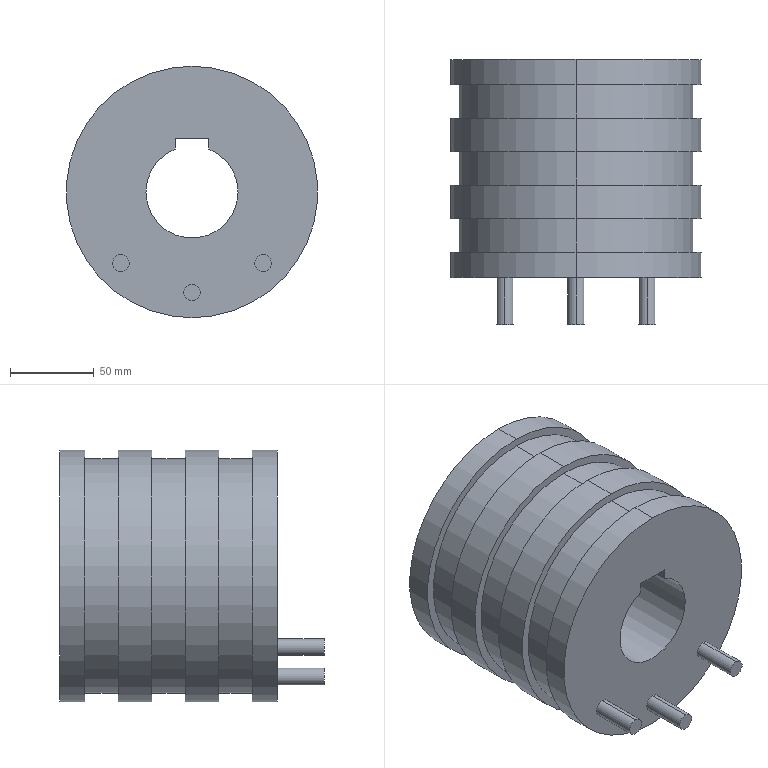Part | SolidWorks | features ICE 2, Revolution 1 | 1 solid | 35 faces | box 150 x 158 x 150 mm | volume 1845061 mm3 | cylinder 21 | plane 14 | commonest cylinder face diameters 150 x8 10 x6 140 x6 55 x1
STEP:
#1=CARTESIAN_POINT('',(42.425,-28.,-47.428));
#2=VERTEX_POINT('',#1);
#3=CARTESIAN_POINT('',(42.425,-28.,-37.428));
#4=VERTEX_POINT('',#3);
#5=CARTESIAN_POINT('',(42.425,-28.,-42.428));
#6=DIRECTION('',(0.,-1.,0.));
#7=DIRECTION('',(0.,0.,-1.));
#8=AXIS2_PLACEMENT_3D('',#5,#6,#7);
#9=CIRCLE('',#8,5.);
#10=EDGE_CURVE('',#2,#4,#9,.T.);
#11=ORIENTED_EDGE('',*,*,#10,.F.);
#12=CARTESIAN_POINT('',(42.425,0.,-47.428));
#13=VERTEX_POINT('',#12);
#14=CARTESIAN_POINT('',(42.425,-28.,-47.428));
#15=DIRECTION('',(0.,1.,0.));
#16=VECTOR('',#15,1000.);
#17=LINE('',#14,#16);
#18=EDGE_CURVE('',#2,#13,#17,.T.);
#19=ORIENTED_EDGE('',*,*,#18,.T.);
#20=CARTESIAN_POINT('',(42.425,0.,-37.428));
#21=VERTEX_POINT('',#20);
#22=CARTESIAN_POINT('',(42.425,0.,-42.428));
#23=DIRECTION('',(0.,-1.,0.));
#24=DIRECTION('',(0.,0.,-1.));
#25=AXIS2_PLACEMENT_3D('',#22,#23,#24);
#26=CIRCLE('',#25,5.);
#27=EDGE_CURVE('',#13,#21,#26,.T.);
#28=ORIENTED_EDGE('',*,*,#27,.T.);
#29=CARTESIAN_POINT('',(42.425,-28.,-37.428));
#30=DIRECTION('',(0.,1.,0.));
#31=VECTOR('',#30,1000.);
#32=LINE('',#29,#31);
#33=EDGE_CURVE('',#4,#21,#32,.T.);
#34=ORIENTED_EDGE('',*,*,#33,.F.);
#35=EDGE_LOOP('',(#11,#19,#28,#34));
#36=FACE_OUTER_BOUND('',#35,.T.);
#37=CARTESIAN_POINT('',(42.425,-28.,-42.428));
#38=DIRECTION('',(0.,1.,0.));
#39=DIRECTION('',(0.,0.,1.));
#40=AXIS2_PLACEMENT_3D('',#37,#38,#39);
#41=CYLINDRICAL_SURFACE('',#40,5.);
#42=ADVANCED_FACE('',(#36),#41,.T.);
#43=CARTESIAN_POINT('',(0.,-28.,-65.));
#44=VERTEX_POINT('',#43);
#45=CARTESIAN_POINT('',(0.,-28.,-55.));
#46=VERTEX_POINT('',#45);
#47=CARTESIAN_POINT('',(0.,-28.,-60.));
#48=DIRECTION('',(0.,-1.,0.));
#49=DIRECTION('',(0.,0.,-1.));
#50=AXIS2_PLACEMENT_3D('',#47,#48,#49);
#51=CIRCLE('',#50,5.);
#52=EDGE_CURVE('',#44,#46,#51,.T.);
#53=ORIENTED_EDGE('',*,*,#52,.F.);
#54=CARTESIAN_POINT('',(0.,0.,-65.));
#55=VERTEX_POINT('',#54);
#56=CARTESIAN_POINT('',(0.,-28.,-65.));
#57=DIRECTION('',(0.,1.,0.));
#58=VECTOR('',#57,1000.);
#59=LINE('',#56,#58);
#60=EDGE_CURVE('',#44,#55,#59,.T.);
#61=ORIENTED_EDGE('',*,*,#60,.T.);
#62=CARTESIAN_POINT('',(0.,0.,-55.));
#63=VERTEX_POINT('',#62);
#64=CARTESIAN_POINT('',(0.,0.,-60.));
#65=DIRECTION('',(0.,-1.,0.));
#66=DIRECTION('',(0.,0.,-1.));
#67=AXIS2_PLACEMENT_3D('',#64,#65,#66);
#68=CIRCLE('',#67,5.);
#69=EDGE_CURVE('',#55,#63,#68,.T.);
#70=ORIENTED_EDGE('',*,*,#69,.T.);
#71=CARTESIAN_POINT('',(0.,-28.,-55.));
#72=DIRECTION('',(0.,1.,0.));
#73=VECTOR('',#72,1000.);
#74=LINE('',#71,#73);
#75=EDGE_CURVE('',#46,#63,#74,.T.);
#76=ORIENTED_EDGE('',*,*,#75,.F.);
#77=EDGE_LOOP('',(#53,#61,#70,#76));
#78=FACE_OUTER_BOUND('',#77,.T.);
#79=CARTESIAN_POINT('',(0.,-28.,-60.));
#80=DIRECTION('',(0.,1.,0.));
#81=DIRECTION('',(0.,0.,1.));
#82=AXIS2_PLACEMENT_3D('',#79,#80,#81);
#83=CYLINDRICAL_SURFACE('',#82,5.);
#84=ADVANCED_FACE('',(#78),#83,.T.);
#85=CARTESIAN_POINT('',(-42.425,-28.,-47.428));
#86=VERTEX_POINT('',#85);
#87=CARTESIAN_POINT('',(-42.425,-28.,-37.428));
#88=VERTEX_POINT('',#87);
#89=CARTESIAN_POINT('',(-42.425,-28.,-42.428));
#90=DIRECTION('',(0.,-1.,0.));
#91=DIRECTION('',(0.,0.,-1.));
#92=AXIS2_PLACEMENT_3D('',#89,#90,#91);
#93=CIRCLE('',#92,5.);
#94=EDGE_CURVE('',#86,#88,#93,.T.);
#95=ORIENTED_EDGE('',*,*,#94,.F.);
#96=CARTESIAN_POINT('',(-42.425,0.,-47.428));
#97=VERTEX_POINT('',#96);
#98=CARTESIAN_POINT('',(-42.425,-28.,-47.428));
#99=DIRECTION('',(0.,1.,0.));
#100=VECTOR('',#99,1000.);
#101=LINE('',#98,#100);
#102=EDGE_CURVE('',#86,#97,#101,.T.);
#103=ORIENTED_EDGE('',*,*,#102,.T.);
#104=CARTESIAN_POINT('',(-42.425,0.,-37.428));
#105=VERTEX_POINT('',#104);
#106=CARTESIAN_POINT('',(-42.425,0.,-42.428));
#107=DIRECTION('',(0.,-1.,0.));
#108=DIRECTION('',(0.,0.,-1.));
#109=AXIS2_PLACEMENT_3D('',#106,#107,#108);
#110=CIRCLE('',#109,5.);
#111=EDGE_CURVE('',#97,#105,#110,.T.);
#112=ORIENTED_EDGE('',*,*,#111,.T.);
#113=CARTESIAN_POINT('',(-42.425,-28.,-37.428));
#114=DIRECTION('',(0.,1.,0.));
#115=VECTOR('',#114,1000.);
#116=LINE('',#113,#115);
#117=EDGE_CURVE('',#88,#105,#116,.T.);
#118=ORIENTED_EDGE('',*,*,#117,.F.);
#119=EDGE_LOOP('',(#95,#103,#112,#118));
#120=FACE_OUTER_BOUND('',#119,.T.);
#121=CARTESIAN_POINT('',(-42.425,-28.,-42.428));
#122=DIRECTION('',(0.,1.,0.));
#123=DIRECTION('',(0.,0.,1.));
#124=AXIS2_PLACEMENT_3D('',#121,#122,#123);
#125=CYLINDRICAL_SURFACE('',#124,5.);
#126=ADVANCED_FACE('',(#120),#125,.T.);
#127=CARTESIAN_POINT('',(0.,75.,-70.));
#128=VERTEX_POINT('',#127);
#129=CARTESIAN_POINT('',(0.,75.,70.));
#130=VERTEX_POINT('',#129);
#131=CARTESIAN_POINT('',(0.,75.,0.));
#132=DIRECTION('',(0.,-1.,0.));
#133=DIRECTION('',(0.,0.,-1.));
#134=AXIS2_PLACEMENT_3D('',#131,#132,#133);
#135=CIRCLE('',#134,70.);
#136=EDGE_CURVE('',#128,#130,#135,.T.);
#137=ORIENTED_EDGE('',*,*,#136,.T.);
#138=CARTESIAN_POINT('',(0.,55.,70.));
#139=VERTEX_POINT('',#138);
#140=CARTESIAN_POINT('',(0.,0.,70.));
#141=DIRECTION('',(0.,-1.,0.));
#142=VECTOR('',#141,1000.);
#143=LINE('',#140,#142);
#144=EDGE_CURVE('',#130,#139,#143,.T.);
#145=ORIENTED_EDGE('',*,*,#144,.T.);
#146=CARTESIAN_POINT('',(0.,55.,-70.));
#147=VERTEX_POINT('',#146);
#148=CARTESIAN_POINT('',(0.,55.,0.));
#149=DIRECTION('',(0.,-1.,0.));
#150=DIRECTION('',(0.,0.,-1.));
#151=AXIS2_PLACEMENT_3D('',#148,#149,#150);
#152=CIRCLE('',#151,70.);
#153=EDGE_CURVE('',#147,#139,#152,.T.);
#154=ORIENTED_EDGE('',*,*,#153,.F.);
#155=CARTESIAN_POINT('',(0.,0.,-70.));
#156=DIRECTION('',(0.,-1.,0.));
#157=VECTOR('',#156,1000.);
#158=LINE('',#155,#157);
#159=EDGE_CURVE('',#128,#147,#158,.T.);
#160=ORIENTED_EDGE('',*,*,#159,.F.);
#161=EDGE_LOOP('',(#137,#145,#154,#160));
#162=FACE_OUTER_BOUND('',#161,.T.);
#163=CARTESIAN_POINT('',(0.,0.,0.));
#164=DIRECTION('',(0.,-1.,0.));
#165=DIRECTION('',(0.,0.,-1.));
#166=AXIS2_PLACEMENT_3D('',#163,#164,#165);
#167=CYLINDRICAL_SURFACE('',#166,70.);
#168=ADVANCED_FACE('',(#162),#167,.T.);
#169=CARTESIAN_POINT('',(0.,55.,-75.));
#170=VERTEX_POINT('',#169);
#171=CARTESIAN_POINT('',(0.,55.,75.));
#172=VERTEX_POINT('',#171);
#173=CARTESIAN_POINT('',(0.,55.,0.));
#174=DIRECTION('',(0.,-1.,0.));
#175=DIRECTION('',(0.,0.,-1.));
#176=AXIS2_PLACEMENT_3D('',#173,#174,#175);
#177=CIRCLE('',#176,75.);
#178=EDGE_CURVE('',#170,#172,#177,.T.);
#179=ORIENTED_EDGE('',*,*,#178,.T.);
#180=CARTESIAN_POINT('',(0.,35.,75.));
#181=VERTEX_POINT('',#180);
#182=CARTESIAN_POINT('',(0.,0.,75.));
#183=DIRECTION('',(0.,-1.,0.));
#184=VECTOR('',#183,1000.);
#185=LINE('',#182,#184);
#186=EDGE_CURVE('',#172,#181,#185,.T.);
#187=ORIENTED_EDGE('',*,*,#186,.T.);
#188=CARTESIAN_POINT('',(0.,35.,-75.));
#189=VERTEX_POINT('',#188);
#190=CARTESIAN_POINT('',(0.,35.,0.));
#191=DIRECTION('',(0.,-1.,0.));
#192=DIRECTION('',(0.,0.,-1.));
#193=AXIS2_PLACEMENT_3D('',#190,#191,#192);
#194=CIRCLE('',#193,75.);
#195=EDGE_CURVE('',#189,#181,#194,.T.);
#196=ORIENTED_EDGE('',*,*,#195,.F.);
#197=CARTESIAN_POINT('',(0.,0.,-75.));
#198=DIRECTION('',(0.,-1.,0.));
#199=VECTOR('',#198,1000.);
#200=LINE('',#197,#199);
#201=EDGE_CURVE('',#170,#189,#200,.T.);
#202=ORIENTED_EDGE('',*,*,#201,.F.);
#203=EDGE_LOOP('',(#179,#187,#196,#202));
#204=FACE_OUTER_BOUND('',#203,.T.);
#205=CARTESIAN_POINT('',(0.,0.,0.));
#206=DIRECTION('',(0.,-1.,0.));
#207=DIRECTION('',(0.,0.,-1.));
#208=AXIS2_PLACEMENT_3D('',#205,#206,#207);
#209=CYLINDRICAL_SURFACE('',#208,75.);
#210=ADVANCED_FACE('',(#204),#209,.T.);
#211=CARTESIAN_POINT('',(0.,35.,-70.));
#212=VERTEX_POINT('',#211);
#213=CARTESIAN_POINT('',(0.,35.,70.));
#214=VERTEX_POINT('',#213);
#215=CARTESIAN_POINT('',(0.,35.,0.));
#216=DIRECTION('',(0.,-1.,0.));
#217=DIRECTION('',(0.,0.,-1.));
#218=AXIS2_PLACEMENT_3D('',#215,#216,#217);
#219=CIRCLE('',#218,70.);
#220=EDGE_CURVE('',#212,#214,#219,.T.);
#221=ORIENTED_EDGE('',*,*,#220,.T.);
#222=CARTESIAN_POINT('',(0.,15.,70.));
#223=VERTEX_POINT('',#222);
#224=CARTESIAN_POINT('',(0.,0.,70.));
#225=DIRECTION('',(0.,-1.,0.));
#226=VECTOR('',#225,1000.);
#227=LINE('',#224,#226);
#228=EDGE_CURVE('',#214,#223,#227,.T.);
#229=ORIENTED_EDGE('',*,*,#228,.T.);
#230=CARTESIAN_POINT('',(0.,15.,-70.));
#231=VERTEX_POINT('',#230);
#232=CARTESIAN_POINT('',(0.,15.,0.));
#233=DIRECTION('',(0.,-1.,0.));
#234=DIRECTION('',(0.,0.,-1.));
#235=AXIS2_PLACEMENT_3D('',#232,#233,#234);
#236=CIRCLE('',#235,70.);
#237=EDGE_CURVE('',#231,#223,#236,.T.);
#238=ORIENTED_EDGE('',*,*,#237,.F.);
#239=CARTESIAN_POINT('',(0.,0.,-70.));
#240=DIRECTION('',(0.,-1.,0.));
#241=VECTOR('',#240,1000.);
#242=LINE('',#239,#241);
#243=EDGE_CURVE('',#212,#231,#242,.T.);
#244=ORIENTED_EDGE('',*,*,#243,.F.);
#245=EDGE_LOOP('',(#221,#229,#238,#244));
#246=FACE_OUTER_BOUND('',#245,.T.);
#247=CARTESIAN_POINT('',(0.,0.,0.));
#248=DIRECTION('',(0.,-1.,0.));
#249=DIRECTION('',(0.,0.,-1.));
#250=AXIS2_PLACEMENT_3D('',#247,#248,#249);
#251=CYLINDRICAL_SURFACE('',#250,70.);
#252=ADVANCED_FACE('',(#246),#251,.T.);
#253=CARTESIAN_POINT('',(0.,15.,-75.));
#254=VERTEX_POINT('',#253);
#255=CARTESIAN_POINT('',(0.,15.,75.));
#256=VERTEX_POINT('',#255);
#257=CARTESIAN_POINT('',(0.,15.,0.));
#258=DIRECTION('',(0.,-1.,0.));
#259=DIRECTION('',(0.,0.,-1.));
#260=AXIS2_PLACEMENT_3D('',#257,#258,#259);
#261=CIRCLE('',#260,75.);
#262=EDGE_CURVE('',#254,#256,#261,.T.);
#263=ORIENTED_EDGE('',*,*,#262,.T.);
#264=CARTESIAN_POINT('',(0.,0.,75.));
#265=VERTEX_POINT('',#264);
#266=CARTESIAN_POINT('',(0.,0.,75.));
#267=DIRECTION('',(0.,-1.,0.));
#268=VECTOR('',#267,1000.);
#269=LINE('',#266,#268);
#270=EDGE_CURVE('',#256,#265,#269,.T.);
#271=ORIENTED_EDGE('',*,*,#270,.T.);
#272=CARTESIAN_POINT('',(0.,0.,-75.));
#273=VERTEX_POINT('',#272);
#274=CARTESIAN_POINT('',(0.,0.,0.));
#275=DIRECTION('',(0.,-1.,0.));
#276=DIRECTION('',(0.,0.,-1.));
#277=AXIS2_PLACEMENT_3D('',#274,#275,#276);
#278=CIRCLE('',#277,75.);
#279=EDGE_CURVE('',#273,#265,#278,.T.);
#280=ORIENTED_EDGE('',*,*,#279,.F.);
#281=CARTESIAN_POINT('',(0.,0.,-75.));
#282=DIRECTION('',(0.,-1.,0.));
#283=VECTOR('',#282,1000.);
#284=LINE('',#281,#283);
#285=EDGE_CURVE('',#254,#273,#284,.T.);
#286=ORIENTED_EDGE('',*,*,#285,.F.);
#287=EDGE_LOOP('',(#263,#271,#280,#286));
#288=FACE_OUTER_BOUND('',#287,.T.);
#289=CARTESIAN_POINT('',(0.,0.,0.));
#290=DIRECTION('',(0.,-1.,0.));
#291=DIRECTION('',(0.,0.,-1.));
#292=AXIS2_PLACEMENT_3D('',#289,#290,#291);
#293=CYLINDRICAL_SURFACE('',#292,75.);
#294=ADVANCED_FACE('',(#288),#293,.T.);
#295=CARTESIAN_POINT('',(0.,130.,-75.));
#296=VERTEX_POINT('',#295);
#297=CARTESIAN_POINT('',(0.,130.,75.));
#298=VERTEX_POINT('',#297);
#299=CARTESIAN_POINT('',(0.,130.,0.));
#300=DIRECTION('',(0.,-1.,0.));
#301=DIRECTION('',(0.,0.,-1.));
#302=AXIS2_PLACEMENT_3D('',#299,#300,#301);
#303=CIRCLE('',#302,75.);
#304=EDGE_CURVE('',#296,#298,#303,.T.);
#305=ORIENTED_EDGE('',*,*,#304,.T.);
#306=CARTESIAN_POINT('',(0.,115.,75.));
#307=VERTEX_POINT('',#306);
#308=CARTESIAN_POINT('',(0.,0.,75.));
#309=DIRECTION('',(0.,-1.,0.));
#310=VECTOR('',#309,1000.);
#311=LINE('',#308,#310);
#312=EDGE_CURVE('',#298,#307,#311,.T.);
#313=ORIENTED_EDGE('',*,*,#312,.T.);
#314=CARTESIAN_POINT('',(0.,115.,-75.));
#315=VERTEX_POINT('',#314);
#316=CARTESIAN_POINT('',(0.,115.,0.));
#317=DIRECTION('',(0.,-1.,0.));
#318=DIRECTION('',(0.,0.,-1.));
#319=AXIS2_PLACEMENT_3D('',#316,#317,#318);
#320=CIRCLE('',#319,75.);
#321=EDGE_CURVE('',#315,#307,#320,.T.);
#322=ORIENTED_EDGE('',*,*,#321,.F.);
#323=CARTESIAN_POINT('',(0.,0.,-75.));
#324=DIRECTION('',(0.,-1.,0.));
#325=VECTOR('',#324,1000.);
#326=LINE('',#323,#325);
#327=EDGE_CURVE('',#296,#315,#326,.T.);
#328=ORIENTED_EDGE('',*,*,#327,.F.);
#329=EDGE_LOOP('',(#305,#313,#322,#328));
#330=FACE_OUTER_BOUND('',#329,.T.);
#331=CARTESIAN_POINT('',(0.,0.,0.));
#332=DIRECTION('',(0.,-1.,0.));
#333=DIRECTION('',(0.,0.,-1.));
#334=AXIS2_PLACEMENT_3D('',#331,#332,#333);
#335=CYLINDRICAL_SURFACE('',#334,75.);
#336=ADVANCED_FACE('',(#330),#335,.T.);
#337=CARTESIAN_POINT('',(0.,115.,-70.));
#338=VERTEX_POINT('',#337);
#339=CARTESIAN_POINT('',(0.,115.,70.));
#340=VERTEX_POINT('',#339);
#341=CARTESIAN_POINT('',(0.,115.,0.));
#342=DIRECTION('',(0.,-1.,0.));
#343=DIRECTION('',(0.,0.,-1.));
#344=AXIS2_PLACEMENT_3D('',#341,#342,#343);
#345=CIRCLE('',#344,70.);
#346=EDGE_CURVE('',#338,#340,#345,.T.);
#347=ORIENTED_EDGE('',*,*,#346,.T.);
#348=CARTESIAN_POINT('',(0.,95.,70.));
#349=VERTEX_POINT('',#348);
#350=CARTESIAN_POINT('',(0.,0.,70.));
#351=DIRECTION('',(0.,-1.,0.));
#352=VECTOR('',#351,1000.);
#353=LINE('',#350,#352);
#354=EDGE_CURVE('',#340,#349,#353,.T.);
#355=ORIENTED_EDGE('',*,*,#354,.T.);
#356=CARTESIAN_POINT('',(0.,95.,-70.));
#357=VERTEX_POINT('',#356);
#358=CARTESIAN_POINT('',(0.,95.,0.));
#359=DIRECTION('',(0.,-1.,0.));
#360=DIRECTION('',(0.,0.,-1.));
#361=AXIS2_PLACEMENT_3D('',#358,#359,#360);
#362=CIRCLE('',#361,70.);
#363=EDGE_CURVE('',#357,#349,#362,.T.);
#364=ORIENTED_EDGE('',*,*,#363,.F.);
#365=CARTESIAN_POINT('',(0.,0.,-70.));
#366=DIRECTION('',(0.,-1.,0.));
#367=VECTOR('',#366,1000.);
#368=LINE('',#365,#367);
#369=EDGE_CURVE('',#338,#357,#368,.T.);
#370=ORIENTED_EDGE('',*,*,#369,.F.);
#371=EDGE_LOOP('',(#347,#355,#364,#370));
#372=FACE_OUTER_BOUND('',#371,.T.);
#373=CARTESIAN_POINT('',(0.,0.,0.));
#374=DIRECTION('',(0.,-1.,0.));
#375=DIRECTION('',(0.,0.,-1.));
#376=AXIS2_PLACEMENT_3D('',#373,#374,#375);
#377=CYLINDRICAL_SURFACE('',#376,70.);
#378=ADVANCED_FACE('',(#372),#377,.T.);
#379=CARTESIAN_POINT('',(0.,95.,-75.));
#380=VERTEX_POINT('',#379);
#381=CARTESIAN_POINT('',(0.,95.,75.));
#382=VERTEX_POINT('',#381);
#383=CARTESIAN_POINT('',(0.,95.,0.));
#384=DIRECTION('',(0.,-1.,0.));
#385=DIRECTION('',(0.,0.,-1.));
#386=AXIS2_PLACEMENT_3D('',#383,#384,#385);
#387=CIRCLE('',#386,75.);
#388=EDGE_CURVE('',#380,#382,#387,.T.);
#389=ORIENTED_EDGE('',*,*,#388,.T.);
#390=CARTESIAN_POINT('',(0.,75.,75.));
#391=VERTEX_POINT('',#390);
#392=CARTESIAN_POINT('',(0.,0.,75.));
#393=DIRECTION('',(0.,-1.,0.));
#394=VECTOR('',#393,1000.);
#395=LINE('',#392,#394);
#396=EDGE_CURVE('',#382,#391,#395,.T.);
#397=ORIENTED_EDGE('',*,*,#396,.T.);
#398=CARTESIAN_POINT('',(0.,75.,-75.));
#399=VERTEX_POINT('',#398);
#400=CARTESIAN_POINT('',(0.,75.,0.));
#401=DIRECTION('',(0.,-1.,0.));
#402=DIRECTION('',(0.,0.,-1.));
#403=AXIS2_PLACEMENT_3D('',#400,#401,#402);
#404=CIRCLE('',#403,75.);
#405=EDGE_CURVE('',#399,#391,#404,.T.);
#406=ORIENTED_EDGE('',*,*,#405,.F.);
#407=CARTESIAN_POINT('',(0.,0.,-75.));
#408=DIRECTION('',(0.,-1.,0.));
#409=VECTOR('',#408,1000.);
#410=LINE('',#407,#409);
#411=EDGE_CURVE('',#380,#399,#410,.T.);
#412=ORIENTED_EDGE('',*,*,#411,.F.);
#413=EDGE_LOOP('',(#389,#397,#406,#412));
#414=FACE_OUTER_BOUND('',#413,.T.);
#415=CARTESIAN_POINT('',(0.,0.,0.));
#416=DIRECTION('',(0.,-1.,0.));
#417=DIRECTION('',(0.,0.,-1.));
#418=AXIS2_PLACEMENT_3D('',#415,#416,#417);
#419=CYLINDRICAL_SURFACE('',#418,75.);
#420=ADVANCED_FACE('',(#414),#419,.T.);
#421=ORIENTED_EDGE('',*,*,#396,.F.);
#422=CARTESIAN_POINT('',(0.,95.,0.));
#423=DIRECTION('',(0.,-1.,0.));
#424=DIRECTION('',(0.,0.,-1.));
#425=AXIS2_PLACEMENT_3D('',#422,#423,#424);
#426=CIRCLE('',#425,75.);
#427=EDGE_CURVE('',#382,#380,#426,.T.);
#428=ORIENTED_EDGE('',*,*,#427,.T.);
#429=ORIENTED_EDGE('',*,*,#411,.T.);
#430=CARTESIAN_POINT('',(0.,75.,0.));
#431=DIRECTION('',(0.,-1.,0.));
#432=DIRECTION('',(0.,0.,-1.));
#433=AXIS2_PLACEMENT_3D('',#430,#431,#432);
#434=CIRCLE('',#433,75.);
#435=EDGE_CURVE('',#391,#399,#434,.T.);
#436=ORIENTED_EDGE('',*,*,#435,.F.);
#437=EDGE_LOOP('',(#421,#428,#429,#436));
#438=FACE_OUTER_BOUND('',#437,.T.);
#439=CARTESIAN_POINT('',(0.,0.,0.));
#440=DIRECTION('',(0.,-1.,0.));
#441=DIRECTION('',(0.,0.,-1.));
#442=AXIS2_PLACEMENT_3D('',#439,#440,#441);
#443=CYLINDRICAL_SURFACE('',#442,75.);
#444=ADVANCED_FACE('',(#438),#443,.T.);
#445=ORIENTED_EDGE('',*,*,#363,.T.);
#446=CARTESIAN_POINT('',(0.,95.,0.));
#447=DIRECTION('',(0.,-1.,0.));
#448=DIRECTION('',(0.,0.,-1.));
#449=AXIS2_PLACEMENT_3D('',#446,#447,#448);
#450=CIRCLE('',#449,70.);
#451=EDGE_CURVE('',#349,#357,#450,.T.);
#452=ORIENTED_EDGE('',*,*,#451,.T.);
#453=EDGE_LOOP('',(#445,#452));
#454=FACE_BOUND('',#453,.T.);
#455=ORIENTED_EDGE('',*,*,#388,.F.);
#456=ORIENTED_EDGE('',*,*,#427,.F.);
#457=EDGE_LOOP('',(#455,#456));
#458=FACE_OUTER_BOUND('',#457,.T.);
#459=CARTESIAN_POINT('',(0.,95.,0.));
#460=DIRECTION('',(0.,1.,0.));
#461=DIRECTION('',(0.,0.,1.));
#462=AXIS2_PLACEMENT_3D('',#459,#460,#461);
#463=PLANE('',#462);
#464=ADVANCED_FACE('',(#454,#458),#463,.T.);
#465=ORIENTED_EDGE('',*,*,#354,.F.);
#466=CARTESIAN_POINT('',(0.,115.,0.));
#467=DIRECTION('',(0.,-1.,0.));
#468=DIRECTION('',(0.,0.,-1.));
#469=AXIS2_PLACEMENT_3D('',#466,#467,#468);
#470=CIRCLE('',#469,70.);
#471=EDGE_CURVE('',#340,#338,#470,.T.);
#472=ORIENTED_EDGE('',*,*,#471,.T.);
#473=ORIENTED_EDGE('',*,*,#369,.T.);
#474=ORIENTED_EDGE('',*,*,#451,.F.);
#475=EDGE_LOOP('',(#465,#472,#473,#474));
#476=FACE_OUTER_BOUND('',#475,.T.);
#477=CARTESIAN_POINT('',(0.,0.,0.));
#478=DIRECTION('',(0.,-1.,0.));
#479=DIRECTION('',(0.,0.,-1.));
#480=AXIS2_PLACEMENT_3D('',#477,#478,#479);
#481=CYLINDRICAL_SURFACE('',#480,70.);
#482=ADVANCED_FACE('',(#476),#481,.T.);
#483=ORIENTED_EDGE('',*,*,#346,.F.);
#484=ORIENTED_EDGE('',*,*,#471,.F.);
#485=EDGE_LOOP('',(#483,#484));
#486=FACE_BOUND('',#485,.T.);
#487=ORIENTED_EDGE('',*,*,#321,.T.);
#488=CARTESIAN_POINT('',(0.,115.,0.));
#489=DIRECTION('',(0.,-1.,0.));
#490=DIRECTION('',(0.,0.,-1.));
#491=AXIS2_PLACEMENT_3D('',#488,#489,#490);
#492=CIRCLE('',#491,75.);
#493=EDGE_CURVE('',#307,#315,#492,.T.);
#494=ORIENTED_EDGE('',*,*,#493,.T.);
#495=EDGE_LOOP('',(#487,#494));
#496=FACE_OUTER_BOUND('',#495,.T.);
#497=CARTESIAN_POINT('',(0.,115.,0.));
#498=DIRECTION('',(0.,1.,0.));
#499=DIRECTION('',(0.,0.,1.));
#500=AXIS2_PLACEMENT_3D('',#497,#498,#499);
#501=PLANE('',#500);
#502=ADVANCED_FACE('',(#486,#496),#501,.F.);
#503=ORIENTED_EDGE('',*,*,#312,.F.);
#504=CARTESIAN_POINT('',(0.,130.,0.));
#505=DIRECTION('',(0.,-1.,0.));
#506=DIRECTION('',(0.,0.,-1.));
#507=AXIS2_PLACEMENT_3D('',#504,#505,#506);
#508=CIRCLE('',#507,75.);
#509=EDGE_CURVE('',#298,#296,#508,.T.);
#510=ORIENTED_EDGE('',*,*,#509,.T.);
#511=ORIENTED_EDGE('',*,*,#327,.T.);
#512=ORIENTED_EDGE('',*,*,#493,.F.);
#513=EDGE_LOOP('',(#503,#510,#511,#512));
#514=FACE_OUTER_BOUND('',#513,.T.);
#515=CARTESIAN_POINT('',(0.,0.,0.));
#516=DIRECTION('',(0.,-1.,0.));
#517=DIRECTION('',(0.,0.,-1.));
#518=AXIS2_PLACEMENT_3D('',#515,#516,#517);
#519=CYLINDRICAL_SURFACE('',#518,75.);
#520=ADVANCED_FACE('',(#514),#519,.T.);
#521=CARTESIAN_POINT('',(-10.,130.,32.));
#522=VERTEX_POINT('',#521);
#523=CARTESIAN_POINT('',(-10.,130.,25.617));
#524=VERTEX_POINT('',#523);
#525=CARTESIAN_POINT('',(-10.,130.,32.));
#526=DIRECTION('',(0.,0.,-1.));
#527=VECTOR('',#526,1000.);
#528=LINE('',#525,#527);
#529=EDGE_CURVE('',#522,#524,#528,.T.);
#530=ORIENTED_EDGE('',*,*,#529,.T.);
#531=CARTESIAN_POINT('',(10.,130.,25.617));
#532=VERTEX_POINT('',#531);
#533=CARTESIAN_POINT('',(0.,130.,0.));
#534=DIRECTION('',(0.,1.,0.));
#535=DIRECTION('',(0.,0.,1.));
#536=AXIS2_PLACEMENT_3D('',#533,#534,#535);
#537=CIRCLE('',#536,27.5);
#538=EDGE_CURVE('',#532,#524,#537,.T.);
#539=ORIENTED_EDGE('',*,*,#538,.F.);
#540=CARTESIAN_POINT('',(10.,130.,32.));
#541=VERTEX_POINT('',#540);
#542=CARTESIAN_POINT('',(10.,130.,32.));
#543=DIRECTION('',(0.,0.,-1.));
#544=VECTOR('',#543,1000.);
#545=LINE('',#542,#544);
#546=EDGE_CURVE('',#541,#532,#545,.T.);
#547=ORIENTED_EDGE('',*,*,#546,.F.);
#548=CARTESIAN_POINT('',(-10.,130.,32.));
#549=DIRECTION('',(1.,0.,0.));
#550=VECTOR('',#549,1000.);
#551=LINE('',#548,#550);
#552=EDGE_CURVE('',#522,#541,#551,.T.);
#553=ORIENTED_EDGE('',*,*,#552,.F.);
#554=EDGE_LOOP('',(#530,#539,#547,#553));
#555=FACE_BOUND('',#554,.T.);
#556=ORIENTED_EDGE('',*,*,#304,.F.);
#557=ORIENTED_EDGE('',*,*,#509,.F.);
#558=EDGE_LOOP('',(#556,#557));
#559=FACE_OUTER_BOUND('',#558,.T.);
#560=CARTESIAN_POINT('',(0.,130.,0.));
#561=DIRECTION('',(0.,-1.,0.));
#562=DIRECTION('',(0.,0.,-1.));
#563=AXIS2_PLACEMENT_3D('',#560,#561,#562);
#564=PLANE('',#563);
#565=ADVANCED_FACE('',(#555,#559),#564,.F.);
#566=CARTESIAN_POINT('',(42.425,0.,-42.428));
#567=DIRECTION('',(0.,-1.,0.));
#568=DIRECTION('',(0.,0.,-1.));
#569=AXIS2_PLACEMENT_3D('',#566,#567,#568);
#570=CIRCLE('',#569,5.);
#571=EDGE_CURVE('',#21,#13,#570,.T.);
#572=ORIENTED_EDGE('',*,*,#571,.F.);
#573=ORIENTED_EDGE('',*,*,#27,.F.);
#574=EDGE_LOOP('',(#572,#573));
#575=FACE_BOUND('',#574,.T.);
#576=CARTESIAN_POINT('',(0.,0.,-60.));
#577=DIRECTION('',(0.,-1.,0.));
#578=DIRECTION('',(0.,0.,-1.));
#579=AXIS2_PLACEMENT_3D('',#576,#577,#578);
#580=CIRCLE('',#579,5.);
#581=EDGE_CURVE('',#63,#55,#580,.T.);
#582=ORIENTED_EDGE('',*,*,#581,.F.);
#583=ORIENTED_EDGE('',*,*,#69,.F.);
#584=EDGE_LOOP('',(#582,#583));
#585=FACE_BOUND('',#584,.T.);
#586=CARTESIAN_POINT('',(-42.425,0.,-42.428));
#587=DIRECTION('',(0.,-1.,0.));
#588=DIRECTION('',(0.,0.,-1.));
#589=AXIS2_PLACEMENT_3D('',#586,#587,#588);
#590=CIRCLE('',#589,5.);
#591=EDGE_CURVE('',#105,#97,#590,.T.);
#592=ORIENTED_EDGE('',*,*,#591,.F.);
#593=ORIENTED_EDGE('',*,*,#111,.F.);
#594=EDGE_LOOP('',(#592,#593));
#595=FACE_BOUND('',#594,.T.);
#596=CARTESIAN_POINT('',(10.,0.,25.617));
#597=VERTEX_POINT('',#596);
#598=CARTESIAN_POINT('',(-10.,0.,25.617));
#599=VERTEX_POINT('',#598);
#600=CARTESIAN_POINT('',(0.,0.,0.));
#601=DIRECTION('',(0.,1.,0.));
#602=DIRECTION('',(0.,0.,1.));
#603=AXIS2_PLACEMENT_3D('',#600,#601,#602);
#604=CIRCLE('',#603,27.5);
#605=EDGE_CURVE('',#597,#599,#604,.T.);
#606=ORIENTED_EDGE('',*,*,#605,.T.);
#607=CARTESIAN_POINT('',(-10.,0.,32.));
#608=VERTEX_POINT('',#607);
#609=CARTESIAN_POINT('',(-10.,0.,32.));
#610=DIRECTION('',(0.,0.,-1.));
#611=VECTOR('',#610,1000.);
#612=LINE('',#609,#611);
#613=EDGE_CURVE('',#608,#599,#612,.T.);
#614=ORIENTED_EDGE('',*,*,#613,.F.);
#615=CARTESIAN_POINT('',(10.,0.,32.));
#616=VERTEX_POINT('',#615);
#617=CARTESIAN_POINT('',(-10.,0.,32.));
#618=DIRECTION('',(1.,0.,0.));
#619=VECTOR('',#618,1000.);
#620=LINE('',#617,#619);
#621=EDGE_CURVE('',#608,#616,#620,.T.);
#622=ORIENTED_EDGE('',*,*,#621,.T.);
#623=CARTESIAN_POINT('',(10.,0.,32.));
#624=DIRECTION('',(0.,0.,-1.));
#625=VECTOR('',#624,1000.);
#626=LINE('',#623,#625);
#627=EDGE_CURVE('',#616,#597,#626,.T.);
#628=ORIENTED_EDGE('',*,*,#627,.T.);
#629=EDGE_LOOP('',(#606,#614,#622,#628));
#630=FACE_BOUND('',#629,.T.);
#631=ORIENTED_EDGE('',*,*,#279,.T.);
#632=CARTESIAN_POINT('',(0.,0.,0.));
#633=DIRECTION('',(0.,-1.,0.));
#634=DIRECTION('',(0.,0.,-1.));
#635=AXIS2_PLACEMENT_3D('',#632,#633,#634);
#636=CIRCLE('',#635,75.);
#637=EDGE_CURVE('',#265,#273,#636,.T.);
#638=ORIENTED_EDGE('',*,*,#637,.T.);
#639=EDGE_LOOP('',(#631,#638));
#640=FACE_OUTER_BOUND('',#639,.T.);
#641=CARTESIAN_POINT('',(0.,0.,0.));
#642=DIRECTION('',(0.,-1.,0.));
#643=DIRECTION('',(0.,0.,-1.));
#644=AXIS2_PLACEMENT_3D('',#641,#642,#643);
#645=PLANE('',#644);
#646=ADVANCED_FACE('',(#575,#585,#595,#630,#640),#645,.T.);
#647=ORIENTED_EDGE('',*,*,#270,.F.);
#648=CARTESIAN_POINT('',(0.,15.,0.));
#649=DIRECTION('',(0.,-1.,0.));
#650=DIRECTION('',(0.,0.,-1.));
#651=AXIS2_PLACEMENT_3D('',#648,#649,#650);
#652=CIRCLE('',#651,75.);
#653=EDGE_CURVE('',#256,#254,#652,.T.);
#654=ORIENTED_EDGE('',*,*,#653,.T.);
#655=ORIENTED_EDGE('',*,*,#285,.T.);
#656=ORIENTED_EDGE('',*,*,#637,.F.);
#657=EDGE_LOOP('',(#647,#654,#655,#656));
#658=FACE_OUTER_BOUND('',#657,.T.);
#659=CARTESIAN_POINT('',(0.,0.,0.));
#660=DIRECTION('',(0.,-1.,0.));
#661=DIRECTION('',(0.,0.,-1.));
#662=AXIS2_PLACEMENT_3D('',#659,#660,#661);
#663=CYLINDRICAL_SURFACE('',#662,75.);
#664=ADVANCED_FACE('',(#658),#663,.T.);
#665=ORIENTED_EDGE('',*,*,#237,.T.);
#666=CARTESIAN_POINT('',(0.,15.,0.));
#667=DIRECTION('',(0.,-1.,0.));
#668=DIRECTION('',(0.,0.,-1.));
#669=AXIS2_PLACEMENT_3D('',#666,#667,#668);
#670=CIRCLE('',#669,70.);
#671=EDGE_CURVE('',#223,#231,#670,.T.);
#672=ORIENTED_EDGE('',*,*,#671,.T.);
#673=EDGE_LOOP('',(#665,#672));
#674=FACE_BOUND('',#673,.T.);
#675=ORIENTED_EDGE('',*,*,#262,.F.);
#676=ORIENTED_EDGE('',*,*,#653,.F.);
#677=EDGE_LOOP('',(#675,#676));
#678=FACE_OUTER_BOUND('',#677,.T.);
#679=CARTESIAN_POINT('',(0.,15.,0.));
#680=DIRECTION('',(0.,1.,0.));
#681=DIRECTION('',(0.,0.,1.));
#682=AXIS2_PLACEMENT_3D('',#679,#680,#681);
#683=PLANE('',#682);
#684=ADVANCED_FACE('',(#674,#678),#683,.T.);
#685=ORIENTED_EDGE('',*,*,#228,.F.);
#686=CARTESIAN_POINT('',(0.,35.,0.));
#687=DIRECTION('',(0.,-1.,0.));
#688=DIRECTION('',(0.,0.,-1.));
#689=AXIS2_PLACEMENT_3D('',#686,#687,#688);
#690=CIRCLE('',#689,70.);
#691=EDGE_CURVE('',#214,#212,#690,.T.);
#692=ORIENTED_EDGE('',*,*,#691,.T.);
#693=ORIENTED_EDGE('',*,*,#243,.T.);
#694=ORIENTED_EDGE('',*,*,#671,.F.);
#695=EDGE_LOOP('',(#685,#692,#693,#694));
#696=FACE_OUTER_BOUND('',#695,.T.);
#697=CARTESIAN_POINT('',(0.,0.,0.));
#698=DIRECTION('',(0.,-1.,0.));
#699=DIRECTION('',(0.,0.,-1.));
#700=AXIS2_PLACEMENT_3D('',#697,#698,#699);
#701=CYLINDRICAL_SURFACE('',#700,70.);
#702=ADVANCED_FACE('',(#696),#701,.T.);
#703=ORIENTED_EDGE('',*,*,#220,.F.);
#704=ORIENTED_EDGE('',*,*,#691,.F.);
#705=EDGE_LOOP('',(#703,#704));
#706=FACE_BOUND('',#705,.T.);
#707=ORIENTED_EDGE('',*,*,#195,.T.);
#708=CARTESIAN_POINT('',(0.,35.,0.));
#709=DIRECTION('',(0.,-1.,0.));
#710=DIRECTION('',(0.,0.,-1.));
#711=AXIS2_PLACEMENT_3D('',#708,#709,#710);
#712=CIRCLE('',#711,75.);
#713=EDGE_CURVE('',#181,#189,#712,.T.);
#714=ORIENTED_EDGE('',*,*,#713,.T.);
#715=EDGE_LOOP('',(#707,#714));
#716=FACE_OUTER_BOUND('',#715,.T.);
#717=CARTESIAN_POINT('',(0.,35.,0.));
#718=DIRECTION('',(0.,1.,0.));
#719=DIRECTION('',(0.,0.,1.));
#720=AXIS2_PLACEMENT_3D('',#717,#718,#719);
#721=PLANE('',#720);
#722=ADVANCED_FACE('',(#706,#716),#721,.F.);
#723=ORIENTED_EDGE('',*,*,#186,.F.);
#724=CARTESIAN_POINT('',(0.,55.,0.));
#725=DIRECTION('',(0.,-1.,0.));
#726=DIRECTION('',(0.,0.,-1.));
#727=AXIS2_PLACEMENT_3D('',#724,#725,#726);
#728=CIRCLE('',#727,75.);
#729=EDGE_CURVE('',#172,#170,#728,.T.);
#730=ORIENTED_EDGE('',*,*,#729,.T.);
#731=ORIENTED_EDGE('',*,*,#201,.T.);
#732=ORIENTED_EDGE('',*,*,#713,.F.);
#733=EDGE_LOOP('',(#723,#730,#731,#732));
#734=FACE_OUTER_BOUND('',#733,.T.);
#735=CARTESIAN_POINT('',(0.,0.,0.));
#736=DIRECTION('',(0.,-1.,0.));
#737=DIRECTION('',(0.,0.,-1.));
#738=AXIS2_PLACEMENT_3D('',#735,#736,#737);
#739=CYLINDRICAL_SURFACE('',#738,75.);
#740=ADVANCED_FACE('',(#734),#739,.T.);
#741=ORIENTED_EDGE('',*,*,#153,.T.);
#742=CARTESIAN_POINT('',(0.,55.,0.));
#743=DIRECTION('',(0.,-1.,0.));
#744=DIRECTION('',(0.,0.,-1.));
#745=AXIS2_PLACEMENT_3D('',#742,#743,#744);
#746=CIRCLE('',#745,70.);
#747=EDGE_CURVE('',#139,#147,#746,.T.);
#748=ORIENTED_EDGE('',*,*,#747,.T.);
#749=EDGE_LOOP('',(#741,#748));
#750=FACE_BOUND('',#749,.T.);
#751=ORIENTED_EDGE('',*,*,#178,.F.);
#752=ORIENTED_EDGE('',*,*,#729,.F.);
#753=EDGE_LOOP('',(#751,#752));
#754=FACE_OUTER_BOUND('',#753,.T.);
#755=CARTESIAN_POINT('',(0.,55.,0.));
#756=DIRECTION('',(0.,1.,0.));
#757=DIRECTION('',(0.,0.,1.));
#758=AXIS2_PLACEMENT_3D('',#755,#756,#757);
#759=PLANE('',#758);
#760=ADVANCED_FACE('',(#750,#754),#759,.T.);
#761=ORIENTED_EDGE('',*,*,#144,.F.);
#762=CARTESIAN_POINT('',(0.,75.,0.));
#763=DIRECTION('',(0.,-1.,0.));
#764=DIRECTION('',(0.,0.,-1.));
#765=AXIS2_PLACEMENT_3D('',#762,#763,#764);
#766=CIRCLE('',#765,70.);
#767=EDGE_CURVE('',#130,#128,#766,.T.);
#768=ORIENTED_EDGE('',*,*,#767,.T.);
#769=ORIENTED_EDGE('',*,*,#159,.T.);
#770=ORIENTED_EDGE('',*,*,#747,.F.);
#771=EDGE_LOOP('',(#761,#768,#769,#770));
#772=FACE_OUTER_BOUND('',#771,.T.);
#773=CARTESIAN_POINT('',(0.,0.,0.));
#774=DIRECTION('',(0.,-1.,0.));
#775=DIRECTION('',(0.,0.,-1.));
#776=AXIS2_PLACEMENT_3D('',#773,#774,#775);
#777=CYLINDRICAL_SURFACE('',#776,70.);
#778=ADVANCED_FACE('',(#772),#777,.T.);
#779=ORIENTED_EDGE('',*,*,#136,.F.);
#780=ORIENTED_EDGE('',*,*,#767,.F.);
#781=EDGE_LOOP('',(#779,#780));
#782=FACE_BOUND('',#781,.T.);
#783=ORIENTED_EDGE('',*,*,#405,.T.);
#784=ORIENTED_EDGE('',*,*,#435,.T.);
#785=EDGE_LOOP('',(#783,#784));
#786=FACE_OUTER_BOUND('',#785,.T.);
#787=CARTESIAN_POINT('',(0.,75.,0.));
#788=DIRECTION('',(0.,1.,0.));
#789=DIRECTION('',(0.,0.,1.));
#790=AXIS2_PLACEMENT_3D('',#787,#788,#789);
#791=PLANE('',#790);
#792=ADVANCED_FACE('',(#782,#786),#791,.F.);
#793=ORIENTED_EDGE('',*,*,#605,.F.);
#794=CARTESIAN_POINT('',(10.,0.,25.617));
#795=DIRECTION('',(0.,1.,0.));
#796=VECTOR('',#795,1000.);
#797=LINE('',#794,#796);
#798=EDGE_CURVE('',#597,#532,#797,.T.);
#799=ORIENTED_EDGE('',*,*,#798,.T.);
#800=ORIENTED_EDGE('',*,*,#538,.T.);
#801=CARTESIAN_POINT('',(-10.,0.,25.617));
#802=DIRECTION('',(0.,1.,0.));
#803=VECTOR('',#802,1000.);
#804=LINE('',#801,#803);
#805=EDGE_CURVE('',#599,#524,#804,.T.);
#806=ORIENTED_EDGE('',*,*,#805,.F.);
#807=EDGE_LOOP('',(#793,#799,#800,#806));
#808=FACE_OUTER_BOUND('',#807,.T.);
#809=CARTESIAN_POINT('',(0.,0.,0.));
#810=DIRECTION('',(0.,1.,0.));
#811=DIRECTION('',(0.,0.,1.));
#812=AXIS2_PLACEMENT_3D('',#809,#810,#811);
#813=CYLINDRICAL_SURFACE('',#812,27.5);
#814=ADVANCED_FACE('',(#808),#813,.F.);
#815=ORIENTED_EDGE('',*,*,#805,.T.);
#816=ORIENTED_EDGE('',*,*,#529,.F.);
#817=CARTESIAN_POINT('',(-10.,0.,32.));
#818=DIRECTION('',(0.,1.,0.));
#819=VECTOR('',#818,1000.);
#820=LINE('',#817,#819);
#821=EDGE_CURVE('',#608,#522,#820,.T.);
#822=ORIENTED_EDGE('',*,*,#821,.F.);
#823=ORIENTED_EDGE('',*,*,#613,.T.);
#824=EDGE_LOOP('',(#815,#816,#822,#823));
#825=FACE_OUTER_BOUND('',#824,.T.);
#826=CARTESIAN_POINT('',(-10.,0.,32.));
#827=DIRECTION('',(1.,0.,0.));
#828=DIRECTION('',(0.,0.,-1.));
#829=AXIS2_PLACEMENT_3D('',#826,#827,#828);
#830=PLANE('',#829);
#831=ADVANCED_FACE('',(#825),#830,.T.);
#832=ORIENTED_EDGE('',*,*,#627,.F.);
#833=CARTESIAN_POINT('',(10.,0.,32.));
#834=DIRECTION('',(0.,1.,0.));
#835=VECTOR('',#834,1000.);
#836=LINE('',#833,#835);
#837=EDGE_CURVE('',#616,#541,#836,.T.);
#838=ORIENTED_EDGE('',*,*,#837,.T.);
#839=ORIENTED_EDGE('',*,*,#546,.T.);
#840=ORIENTED_EDGE('',*,*,#798,.F.);
#841=EDGE_LOOP('',(#832,#838,#839,#840));
#842=FACE_OUTER_BOUND('',#841,.T.);
#843=CARTESIAN_POINT('',(10.,0.,32.));
#844=DIRECTION('',(1.,0.,0.));
#845=DIRECTION('',(0.,0.,-1.));
#846=AXIS2_PLACEMENT_3D('',#843,#844,#845);
#847=PLANE('',#846);
#848=ADVANCED_FACE('',(#842),#847,.F.);
#849=ORIENTED_EDGE('',*,*,#552,.T.);
#850=ORIENTED_EDGE('',*,*,#837,.F.);
#851=ORIENTED_EDGE('',*,*,#621,.F.);
#852=ORIENTED_EDGE('',*,*,#821,.T.);
#853=EDGE_LOOP('',(#849,#850,#851,#852));
#854=FACE_OUTER_BOUND('',#853,.T.);
#855=CARTESIAN_POINT('',(-10.,0.,32.));
#856=DIRECTION('',(0.,0.,1.));
#857=DIRECTION('',(1.,0.,0.));
#858=AXIS2_PLACEMENT_3D('',#855,#856,#857);
#859=PLANE('',#858);
#860=ADVANCED_FACE('',(#854),#859,.F.);
#861=ORIENTED_EDGE('',*,*,#102,.F.);
#862=CARTESIAN_POINT('',(-42.425,-28.,-42.428));
#863=DIRECTION('',(0.,-1.,0.));
#864=DIRECTION('',(0.,0.,-1.));
#865=AXIS2_PLACEMENT_3D('',#862,#863,#864);
#866=CIRCLE('',#865,5.);
#867=EDGE_CURVE('',#88,#86,#866,.T.);
#868=ORIENTED_EDGE('',*,*,#867,.F.);
#869=ORIENTED_EDGE('',*,*,#117,.T.);
#870=ORIENTED_EDGE('',*,*,#591,.T.);
#871=EDGE_LOOP('',(#861,#868,#869,#870));
#872=FACE_OUTER_BOUND('',#871,.T.);
#873=CARTESIAN_POINT('',(-42.425,-28.,-42.428));
#874=DIRECTION('',(0.,1.,0.));
#875=DIRECTION('',(0.,0.,1.));
#876=AXIS2_PLACEMENT_3D('',#873,#874,#875);
#877=CYLINDRICAL_SURFACE('',#876,5.);
#878=ADVANCED_FACE('',(#872),#877,.T.);
#879=ORIENTED_EDGE('',*,*,#867,.T.);
#880=ORIENTED_EDGE('',*,*,#94,.T.);
#881=EDGE_LOOP('',(#879,#880));
#882=FACE_OUTER_BOUND('',#881,.T.);
#883=CARTESIAN_POINT('',(-42.425,-28.,-42.428));
#884=DIRECTION('',(0.,-1.,0.));
#885=DIRECTION('',(0.,0.,-1.));
#886=AXIS2_PLACEMENT_3D('',#883,#884,#885);
#887=PLANE('',#886);
#888=ADVANCED_FACE('',(#882),#887,.T.);
#889=ORIENTED_EDGE('',*,*,#60,.F.);
#890=CARTESIAN_POINT('',(0.,-28.,-60.));
#891=DIRECTION('',(0.,-1.,0.));
#892=DIRECTION('',(0.,0.,-1.));
#893=AXIS2_PLACEMENT_3D('',#890,#891,#892);
#894=CIRCLE('',#893,5.);
#895=EDGE_CURVE('',#46,#44,#894,.T.);
#896=ORIENTED_EDGE('',*,*,#895,.F.);
#897=ORIENTED_EDGE('',*,*,#75,.T.);
#898=ORIENTED_EDGE('',*,*,#581,.T.);
#899=EDGE_LOOP('',(#889,#896,#897,#898));
#900=FACE_OUTER_BOUND('',#899,.T.);
#901=CARTESIAN_POINT('',(0.,-28.,-60.));
#902=DIRECTION('',(0.,1.,0.));
#903=DIRECTION('',(0.,0.,1.));
#904=AXIS2_PLACEMENT_3D('',#901,#902,#903);
#905=CYLINDRICAL_SURFACE('',#904,5.);
#906=ADVANCED_FACE('',(#900),#905,.T.);
#907=ORIENTED_EDGE('',*,*,#895,.T.);
#908=ORIENTED_EDGE('',*,*,#52,.T.);
#909=EDGE_LOOP('',(#907,#908));
#910=FACE_OUTER_BOUND('',#909,.T.);
#911=CARTESIAN_POINT('',(0.,-28.,-60.));
#912=DIRECTION('',(0.,-1.,0.));
#913=DIRECTION('',(0.,0.,-1.));
#914=AXIS2_PLACEMENT_3D('',#911,#912,#913);
#915=PLANE('',#914);
#916=ADVANCED_FACE('',(#910),#915,.T.);
#917=ORIENTED_EDGE('',*,*,#18,.F.);
#918=CARTESIAN_POINT('',(42.425,-28.,-42.428));
#919=DIRECTION('',(0.,-1.,0.));
#920=DIRECTION('',(0.,0.,-1.));
#921=AXIS2_PLACEMENT_3D('',#918,#919,#920);
#922=CIRCLE('',#921,5.);
#923=EDGE_CURVE('',#4,#2,#922,.T.);
#924=ORIENTED_EDGE('',*,*,#923,.F.);
#925=ORIENTED_EDGE('',*,*,#33,.T.);
#926=ORIENTED_EDGE('',*,*,#571,.T.);
#927=EDGE_LOOP('',(#917,#924,#925,#926));
#928=FACE_OUTER_BOUND('',#927,.T.);
#929=CARTESIAN_POINT('',(42.425,-28.,-42.428));
#930=DIRECTION('',(0.,1.,0.));
#931=DIRECTION('',(0.,0.,1.));
#932=AXIS2_PLACEMENT_3D('',#929,#930,#931);
#933=CYLINDRICAL_SURFACE('',#932,5.);
#934=ADVANCED_FACE('',(#928),#933,.T.);
#935=ORIENTED_EDGE('',*,*,#923,.T.);
#936=ORIENTED_EDGE('',*,*,#10,.T.);
#937=EDGE_LOOP('',(#935,#936));
#938=FACE_OUTER_BOUND('',#937,.T.);
#939=CARTESIAN_POINT('',(42.425,-28.,-42.428));
#940=DIRECTION('',(0.,-1.,0.));
#941=DIRECTION('',(0.,0.,-1.));
#942=AXIS2_PLACEMENT_3D('',#939,#940,#941);
#943=PLANE('',#942);
#944=ADVANCED_FACE('',(#938),#943,.T.);
#945=CLOSED_SHELL('',(#42,#84,#126,#168,#210,#252,#294,#336,#378,#420,#444,#464,#482,#502,#520,#565,#646,#664,#684,#702,#722,#740,#760,#778,#792,#814,#831,#848,#860,#878,#888,#906,#916,#934,#944));
#946=MANIFOLD_SOLID_BREP('',#945);
#947=CARTESIAN_POINT('',(0.,0.,0.));
#948=DIRECTION('',(0.,0.,1.));
#949=DIRECTION('',(1.,0.,0.));
#950=AXIS2_PLACEMENT_3D('',#947,#948,#949);
#951=(LENGTH_UNIT()NAMED_UNIT(*)SI_UNIT(.MILLI.,.METRE.));
#952=UNCERTAINTY_MEASURE_WITH_UNIT(LENGTH_MEASURE(0.00001),#951,'','');
#953=(NAMED_UNIT(*)PLANE_ANGLE_UNIT()SI_UNIT($,.RADIAN.));
#954=(NAMED_UNIT(*)SI_UNIT($,.STERADIAN.)SOLID_ANGLE_UNIT());
#955=(GEOMETRIC_REPRESENTATION_CONTEXT(3)GLOBAL_UNCERTAINTY_ASSIGNED_CONTEXT((#952))GLOBAL_UNIT_ASSIGNED_CONTEXT((#951,#953,#954))REPRESENTATION_CONTEXT('',''));
#956=ADVANCED_BREP_SHAPE_REPRESENTATION('',(#946,#950),#955);